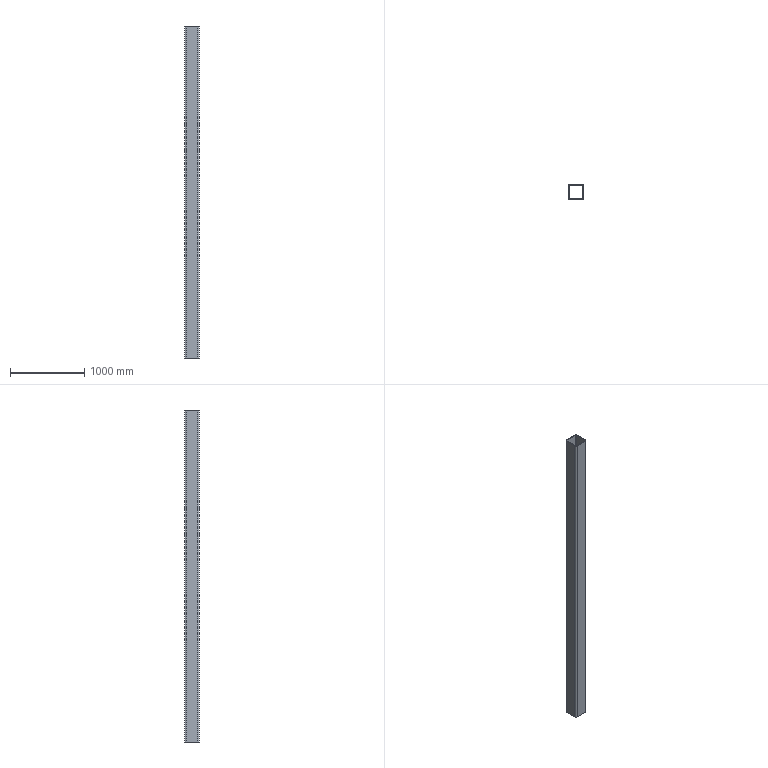Part | SolidWorks | features Extrusion 1 | 1 solid | 18 faces | box 200 x 200 x 4480 mm | volume 26540630 mm3 | plane 10 | cylinder 8 | commonest cylinder face diameters 24 x4 40 x4
STEP:
#1=CARTESIAN_POINT('',(-100.,-80.,4480.));
#2=VERTEX_POINT('',#1);
#3=CARTESIAN_POINT('',(-80.,-100.,4480.));
#4=VERTEX_POINT('',#3);
#5=CARTESIAN_POINT('',(-80.,-80.,4480.));
#6=DIRECTION('',(0.,0.,1.));
#7=DIRECTION('',(1.,0.,0.));
#8=AXIS2_PLACEMENT_3D('',#5,#6,#7);
#9=CIRCLE('',#8,20.);
#10=EDGE_CURVE('',#2,#4,#9,.T.);
#11=ORIENTED_EDGE('',*,*,#10,.T.);
#12=CARTESIAN_POINT('',(80.,-100.,4480.));
#13=VERTEX_POINT('',#12);
#14=CARTESIAN_POINT('',(-80.,-100.,4480.));
#15=DIRECTION('',(1.,0.,0.));
#16=VECTOR('',#15,1000.);
#17=LINE('',#14,#16);
#18=EDGE_CURVE('',#4,#13,#17,.T.);
#19=ORIENTED_EDGE('',*,*,#18,.T.);
#20=CARTESIAN_POINT('',(100.,-80.,4480.));
#21=VERTEX_POINT('',#20);
#22=CARTESIAN_POINT('',(80.,-80.,4480.));
#23=DIRECTION('',(0.,0.,1.));
#24=DIRECTION('',(1.,0.,0.));
#25=AXIS2_PLACEMENT_3D('',#22,#23,#24);
#26=CIRCLE('',#25,20.);
#27=EDGE_CURVE('',#13,#21,#26,.T.);
#28=ORIENTED_EDGE('',*,*,#27,.T.);
#29=CARTESIAN_POINT('',(100.,80.,4480.));
#30=VERTEX_POINT('',#29);
#31=CARTESIAN_POINT('',(100.,80.,4480.));
#32=DIRECTION('',(0.,1.,0.));
#33=VECTOR('',#32,1000.);
#34=LINE('',#31,#33);
#35=EDGE_CURVE('',#21,#30,#34,.T.);
#36=ORIENTED_EDGE('',*,*,#35,.T.);
#37=CARTESIAN_POINT('',(80.,100.,4480.));
#38=VERTEX_POINT('',#37);
#39=CARTESIAN_POINT('',(80.,80.,4480.));
#40=DIRECTION('',(0.,0.,1.));
#41=DIRECTION('',(-1.,0.,0.));
#42=AXIS2_PLACEMENT_3D('',#39,#40,#41);
#43=CIRCLE('',#42,20.);
#44=EDGE_CURVE('',#30,#38,#43,.T.);
#45=ORIENTED_EDGE('',*,*,#44,.T.);
#46=CARTESIAN_POINT('',(-80.,100.,4480.));
#47=VERTEX_POINT('',#46);
#48=CARTESIAN_POINT('',(-80.,100.,4480.));
#49=DIRECTION('',(-1.,0.,0.));
#50=VECTOR('',#49,1000.);
#51=LINE('',#48,#50);
#52=EDGE_CURVE('',#38,#47,#51,.T.);
#53=ORIENTED_EDGE('',*,*,#52,.T.);
#54=CARTESIAN_POINT('',(-100.,80.,4480.));
#55=VERTEX_POINT('',#54);
#56=CARTESIAN_POINT('',(-80.,80.,4480.));
#57=DIRECTION('',(0.,0.,1.));
#58=DIRECTION('',(1.,0.,0.));
#59=AXIS2_PLACEMENT_3D('',#56,#57,#58);
#60=CIRCLE('',#59,20.);
#61=EDGE_CURVE('',#47,#55,#60,.T.);
#62=ORIENTED_EDGE('',*,*,#61,.T.);
#63=CARTESIAN_POINT('',(-100.,80.,4480.));
#64=DIRECTION('',(0.,-1.,0.));
#65=VECTOR('',#64,1000.);
#66=LINE('',#63,#65);
#67=EDGE_CURVE('',#55,#2,#66,.T.);
#68=ORIENTED_EDGE('',*,*,#67,.T.);
#69=EDGE_LOOP('',(#11,#19,#28,#36,#45,#53,#62,#68));
#70=FACE_OUTER_BOUND('',#69,.T.);
#71=CARTESIAN_POINT('',(-92.,80.,4480.));
#72=VERTEX_POINT('',#71);
#73=CARTESIAN_POINT('',(-92.,-80.,4480.));
#74=VERTEX_POINT('',#73);
#75=CARTESIAN_POINT('',(-92.,80.,4480.));
#76=DIRECTION('',(0.,-1.,0.));
#77=VECTOR('',#76,1000.);
#78=LINE('',#75,#77);
#79=EDGE_CURVE('',#72,#74,#78,.T.);
#80=ORIENTED_EDGE('',*,*,#79,.F.);
#81=CARTESIAN_POINT('',(-80.,92.,4480.));
#82=VERTEX_POINT('',#81);
#83=CARTESIAN_POINT('',(-80.,80.,4480.));
#84=DIRECTION('',(0.,0.,1.));
#85=DIRECTION('',(1.,0.,0.));
#86=AXIS2_PLACEMENT_3D('',#83,#84,#85);
#87=CIRCLE('',#86,12.);
#88=EDGE_CURVE('',#82,#72,#87,.T.);
#89=ORIENTED_EDGE('',*,*,#88,.F.);
#90=CARTESIAN_POINT('',(80.,92.,4480.));
#91=VERTEX_POINT('',#90);
#92=CARTESIAN_POINT('',(-80.,92.,4480.));
#93=DIRECTION('',(-1.,0.,0.));
#94=VECTOR('',#93,1000.);
#95=LINE('',#92,#94);
#96=EDGE_CURVE('',#91,#82,#95,.T.);
#97=ORIENTED_EDGE('',*,*,#96,.F.);
#98=CARTESIAN_POINT('',(92.,80.,4480.));
#99=VERTEX_POINT('',#98);
#100=CARTESIAN_POINT('',(80.,80.,4480.));
#101=DIRECTION('',(0.,0.,1.));
#102=DIRECTION('',(-1.,0.,0.));
#103=AXIS2_PLACEMENT_3D('',#100,#101,#102);
#104=CIRCLE('',#103,12.);
#105=EDGE_CURVE('',#99,#91,#104,.T.);
#106=ORIENTED_EDGE('',*,*,#105,.F.);
#107=CARTESIAN_POINT('',(92.,-80.,4480.));
#108=VERTEX_POINT('',#107);
#109=CARTESIAN_POINT('',(92.,80.,4480.));
#110=DIRECTION('',(0.,1.,0.));
#111=VECTOR('',#110,1000.);
#112=LINE('',#109,#111);
#113=EDGE_CURVE('',#108,#99,#112,.T.);
#114=ORIENTED_EDGE('',*,*,#113,.F.);
#115=CARTESIAN_POINT('',(80.,-92.,4480.));
#116=VERTEX_POINT('',#115);
#117=CARTESIAN_POINT('',(80.,-80.,4480.));
#118=DIRECTION('',(0.,0.,1.));
#119=DIRECTION('',(1.,0.,0.));
#120=AXIS2_PLACEMENT_3D('',#117,#118,#119);
#121=CIRCLE('',#120,12.);
#122=EDGE_CURVE('',#116,#108,#121,.T.);
#123=ORIENTED_EDGE('',*,*,#122,.F.);
#124=CARTESIAN_POINT('',(-80.,-92.,4480.));
#125=VERTEX_POINT('',#124);
#126=CARTESIAN_POINT('',(-80.,-92.,4480.));
#127=DIRECTION('',(1.,0.,0.));
#128=VECTOR('',#127,1000.);
#129=LINE('',#126,#128);
#130=EDGE_CURVE('',#125,#116,#129,.T.);
#131=ORIENTED_EDGE('',*,*,#130,.F.);
#132=CARTESIAN_POINT('',(-80.,-80.,4480.));
#133=DIRECTION('',(0.,0.,1.));
#134=DIRECTION('',(1.,0.,0.));
#135=AXIS2_PLACEMENT_3D('',#132,#133,#134);
#136=CIRCLE('',#135,12.);
#137=EDGE_CURVE('',#74,#125,#136,.T.);
#138=ORIENTED_EDGE('',*,*,#137,.F.);
#139=EDGE_LOOP('',(#80,#89,#97,#106,#114,#123,#131,#138));
#140=FACE_BOUND('',#139,.T.);
#141=CARTESIAN_POINT('',(-80.,-80.,4480.));
#142=DIRECTION('',(0.,0.,1.));
#143=DIRECTION('',(1.,0.,0.));
#144=AXIS2_PLACEMENT_3D('',#141,#142,#143);
#145=PLANE('',#144);
#146=ADVANCED_FACE('',(#70,#140),#145,.T.);
#147=CARTESIAN_POINT('',(-100.,-80.,0.));
#148=VERTEX_POINT('',#147);
#149=CARTESIAN_POINT('',(-80.,-100.,0.));
#150=VERTEX_POINT('',#149);
#151=CARTESIAN_POINT('',(-80.,-80.,0.));
#152=DIRECTION('',(0.,0.,1.));
#153=DIRECTION('',(1.,0.,0.));
#154=AXIS2_PLACEMENT_3D('',#151,#152,#153);
#155=CIRCLE('',#154,20.);
#156=EDGE_CURVE('',#148,#150,#155,.T.);
#157=ORIENTED_EDGE('',*,*,#156,.F.);
#158=CARTESIAN_POINT('',(-100.,80.,0.));
#159=VERTEX_POINT('',#158);
#160=CARTESIAN_POINT('',(-100.,80.,0.));
#161=DIRECTION('',(0.,-1.,0.));
#162=VECTOR('',#161,1000.);
#163=LINE('',#160,#162);
#164=EDGE_CURVE('',#159,#148,#163,.T.);
#165=ORIENTED_EDGE('',*,*,#164,.F.);
#166=CARTESIAN_POINT('',(-80.,100.,0.));
#167=VERTEX_POINT('',#166);
#168=CARTESIAN_POINT('',(-80.,80.,0.));
#169=DIRECTION('',(0.,0.,1.));
#170=DIRECTION('',(1.,0.,0.));
#171=AXIS2_PLACEMENT_3D('',#168,#169,#170);
#172=CIRCLE('',#171,20.);
#173=EDGE_CURVE('',#167,#159,#172,.T.);
#174=ORIENTED_EDGE('',*,*,#173,.F.);
#175=CARTESIAN_POINT('',(80.,100.,0.));
#176=VERTEX_POINT('',#175);
#177=CARTESIAN_POINT('',(-80.,100.,0.));
#178=DIRECTION('',(-1.,0.,0.));
#179=VECTOR('',#178,1000.);
#180=LINE('',#177,#179);
#181=EDGE_CURVE('',#176,#167,#180,.T.);
#182=ORIENTED_EDGE('',*,*,#181,.F.);
#183=CARTESIAN_POINT('',(100.,80.,0.));
#184=VERTEX_POINT('',#183);
#185=CARTESIAN_POINT('',(80.,80.,0.));
#186=DIRECTION('',(0.,0.,1.));
#187=DIRECTION('',(-1.,0.,0.));
#188=AXIS2_PLACEMENT_3D('',#185,#186,#187);
#189=CIRCLE('',#188,20.);
#190=EDGE_CURVE('',#184,#176,#189,.T.);
#191=ORIENTED_EDGE('',*,*,#190,.F.);
#192=CARTESIAN_POINT('',(100.,-80.,0.));
#193=VERTEX_POINT('',#192);
#194=CARTESIAN_POINT('',(100.,80.,0.));
#195=DIRECTION('',(0.,1.,0.));
#196=VECTOR('',#195,1000.);
#197=LINE('',#194,#196);
#198=EDGE_CURVE('',#193,#184,#197,.T.);
#199=ORIENTED_EDGE('',*,*,#198,.F.);
#200=CARTESIAN_POINT('',(80.,-100.,0.));
#201=VERTEX_POINT('',#200);
#202=CARTESIAN_POINT('',(80.,-80.,0.));
#203=DIRECTION('',(0.,0.,1.));
#204=DIRECTION('',(1.,0.,0.));
#205=AXIS2_PLACEMENT_3D('',#202,#203,#204);
#206=CIRCLE('',#205,20.);
#207=EDGE_CURVE('',#201,#193,#206,.T.);
#208=ORIENTED_EDGE('',*,*,#207,.F.);
#209=CARTESIAN_POINT('',(-80.,-100.,0.));
#210=DIRECTION('',(1.,0.,0.));
#211=VECTOR('',#210,1000.);
#212=LINE('',#209,#211);
#213=EDGE_CURVE('',#150,#201,#212,.T.);
#214=ORIENTED_EDGE('',*,*,#213,.F.);
#215=EDGE_LOOP('',(#157,#165,#174,#182,#191,#199,#208,#214));
#216=FACE_OUTER_BOUND('',#215,.T.);
#217=CARTESIAN_POINT('',(-80.,92.,0.));
#218=VERTEX_POINT('',#217);
#219=CARTESIAN_POINT('',(-92.,80.,0.));
#220=VERTEX_POINT('',#219);
#221=CARTESIAN_POINT('',(-80.,80.,0.));
#222=DIRECTION('',(0.,0.,1.));
#223=DIRECTION('',(1.,0.,0.));
#224=AXIS2_PLACEMENT_3D('',#221,#222,#223);
#225=CIRCLE('',#224,12.);
#226=EDGE_CURVE('',#218,#220,#225,.T.);
#227=ORIENTED_EDGE('',*,*,#226,.T.);
#228=CARTESIAN_POINT('',(-92.,-80.,0.));
#229=VERTEX_POINT('',#228);
#230=CARTESIAN_POINT('',(-92.,80.,0.));
#231=DIRECTION('',(0.,-1.,0.));
#232=VECTOR('',#231,1000.);
#233=LINE('',#230,#232);
#234=EDGE_CURVE('',#220,#229,#233,.T.);
#235=ORIENTED_EDGE('',*,*,#234,.T.);
#236=CARTESIAN_POINT('',(-80.,-92.,0.));
#237=VERTEX_POINT('',#236);
#238=CARTESIAN_POINT('',(-80.,-80.,0.));
#239=DIRECTION('',(0.,0.,1.));
#240=DIRECTION('',(1.,0.,0.));
#241=AXIS2_PLACEMENT_3D('',#238,#239,#240);
#242=CIRCLE('',#241,12.);
#243=EDGE_CURVE('',#229,#237,#242,.T.);
#244=ORIENTED_EDGE('',*,*,#243,.T.);
#245=CARTESIAN_POINT('',(80.,-92.,0.));
#246=VERTEX_POINT('',#245);
#247=CARTESIAN_POINT('',(-80.,-92.,0.));
#248=DIRECTION('',(1.,0.,0.));
#249=VECTOR('',#248,1000.);
#250=LINE('',#247,#249);
#251=EDGE_CURVE('',#237,#246,#250,.T.);
#252=ORIENTED_EDGE('',*,*,#251,.T.);
#253=CARTESIAN_POINT('',(92.,-80.,0.));
#254=VERTEX_POINT('',#253);
#255=CARTESIAN_POINT('',(80.,-80.,0.));
#256=DIRECTION('',(0.,0.,1.));
#257=DIRECTION('',(1.,0.,0.));
#258=AXIS2_PLACEMENT_3D('',#255,#256,#257);
#259=CIRCLE('',#258,12.);
#260=EDGE_CURVE('',#246,#254,#259,.T.);
#261=ORIENTED_EDGE('',*,*,#260,.T.);
#262=CARTESIAN_POINT('',(92.,80.,0.));
#263=VERTEX_POINT('',#262);
#264=CARTESIAN_POINT('',(92.,80.,0.));
#265=DIRECTION('',(0.,1.,0.));
#266=VECTOR('',#265,1000.);
#267=LINE('',#264,#266);
#268=EDGE_CURVE('',#254,#263,#267,.T.);
#269=ORIENTED_EDGE('',*,*,#268,.T.);
#270=CARTESIAN_POINT('',(80.,92.,0.));
#271=VERTEX_POINT('',#270);
#272=CARTESIAN_POINT('',(80.,80.,0.));
#273=DIRECTION('',(0.,0.,1.));
#274=DIRECTION('',(-1.,0.,0.));
#275=AXIS2_PLACEMENT_3D('',#272,#273,#274);
#276=CIRCLE('',#275,12.);
#277=EDGE_CURVE('',#263,#271,#276,.T.);
#278=ORIENTED_EDGE('',*,*,#277,.T.);
#279=CARTESIAN_POINT('',(-80.,92.,0.));
#280=DIRECTION('',(-1.,0.,0.));
#281=VECTOR('',#280,1000.);
#282=LINE('',#279,#281);
#283=EDGE_CURVE('',#271,#218,#282,.T.);
#284=ORIENTED_EDGE('',*,*,#283,.T.);
#285=EDGE_LOOP('',(#227,#235,#244,#252,#261,#269,#278,#284));
#286=FACE_BOUND('',#285,.T.);
#287=CARTESIAN_POINT('',(-80.,-80.,0.));
#288=DIRECTION('',(0.,0.,1.));
#289=DIRECTION('',(1.,0.,0.));
#290=AXIS2_PLACEMENT_3D('',#287,#288,#289);
#291=PLANE('',#290);
#292=ADVANCED_FACE('',(#216,#286),#291,.F.);
#293=ORIENTED_EDGE('',*,*,#156,.T.);
#294=CARTESIAN_POINT('',(-80.,-100.,4480.));
#295=DIRECTION('',(0.,0.,-1.));
#296=VECTOR('',#295,1000.);
#297=LINE('',#294,#296);
#298=EDGE_CURVE('',#4,#150,#297,.T.);
#299=ORIENTED_EDGE('',*,*,#298,.F.);
#300=ORIENTED_EDGE('',*,*,#10,.F.);
#301=CARTESIAN_POINT('',(-100.,-80.,4480.));
#302=DIRECTION('',(0.,0.,-1.));
#303=VECTOR('',#302,1000.);
#304=LINE('',#301,#303);
#305=EDGE_CURVE('',#2,#148,#304,.T.);
#306=ORIENTED_EDGE('',*,*,#305,.T.);
#307=EDGE_LOOP('',(#293,#299,#300,#306));
#308=FACE_OUTER_BOUND('',#307,.T.);
#309=CARTESIAN_POINT('',(-80.,-80.,4480.));
#310=DIRECTION('',(0.,0.,-1.));
#311=DIRECTION('',(-1.,0.,0.));
#312=AXIS2_PLACEMENT_3D('',#309,#310,#311);
#313=CYLINDRICAL_SURFACE('',#312,20.);
#314=ADVANCED_FACE('',(#308),#313,.T.);
#315=ORIENTED_EDGE('',*,*,#213,.T.);
#316=CARTESIAN_POINT('',(80.,-100.,4480.));
#317=DIRECTION('',(0.,0.,-1.));
#318=VECTOR('',#317,1000.);
#319=LINE('',#316,#318);
#320=EDGE_CURVE('',#13,#201,#319,.T.);
#321=ORIENTED_EDGE('',*,*,#320,.F.);
#322=ORIENTED_EDGE('',*,*,#18,.F.);
#323=ORIENTED_EDGE('',*,*,#298,.T.);
#324=EDGE_LOOP('',(#315,#321,#322,#323));
#325=FACE_OUTER_BOUND('',#324,.T.);
#326=CARTESIAN_POINT('',(-80.,-100.,4480.));
#327=DIRECTION('',(0.,1.,0.));
#328=DIRECTION('',(0.,0.,1.));
#329=AXIS2_PLACEMENT_3D('',#326,#327,#328);
#330=PLANE('',#329);
#331=ADVANCED_FACE('',(#325),#330,.F.);
#332=ORIENTED_EDGE('',*,*,#207,.T.);
#333=CARTESIAN_POINT('',(100.,-80.,4480.));
#334=DIRECTION('',(0.,0.,-1.));
#335=VECTOR('',#334,1000.);
#336=LINE('',#333,#335);
#337=EDGE_CURVE('',#21,#193,#336,.T.);
#338=ORIENTED_EDGE('',*,*,#337,.F.);
#339=ORIENTED_EDGE('',*,*,#27,.F.);
#340=ORIENTED_EDGE('',*,*,#320,.T.);
#341=EDGE_LOOP('',(#332,#338,#339,#340));
#342=FACE_OUTER_BOUND('',#341,.T.);
#343=CARTESIAN_POINT('',(80.,-80.,4480.));
#344=DIRECTION('',(0.,0.,-1.));
#345=DIRECTION('',(-1.,0.,0.));
#346=AXIS2_PLACEMENT_3D('',#343,#344,#345);
#347=CYLINDRICAL_SURFACE('',#346,20.);
#348=ADVANCED_FACE('',(#342),#347,.T.);
#349=ORIENTED_EDGE('',*,*,#198,.T.);
#350=CARTESIAN_POINT('',(100.,80.,4480.));
#351=DIRECTION('',(0.,0.,-1.));
#352=VECTOR('',#351,1000.);
#353=LINE('',#350,#352);
#354=EDGE_CURVE('',#30,#184,#353,.T.);
#355=ORIENTED_EDGE('',*,*,#354,.F.);
#356=ORIENTED_EDGE('',*,*,#35,.F.);
#357=ORIENTED_EDGE('',*,*,#337,.T.);
#358=EDGE_LOOP('',(#349,#355,#356,#357));
#359=FACE_OUTER_BOUND('',#358,.T.);
#360=CARTESIAN_POINT('',(100.,80.,4480.));
#361=DIRECTION('',(-1.,0.,0.));
#362=DIRECTION('',(0.,-1.,0.));
#363=AXIS2_PLACEMENT_3D('',#360,#361,#362);
#364=PLANE('',#363);
#365=ADVANCED_FACE('',(#359),#364,.F.);
#366=ORIENTED_EDGE('',*,*,#190,.T.);
#367=CARTESIAN_POINT('',(80.,100.,4480.));
#368=DIRECTION('',(0.,0.,-1.));
#369=VECTOR('',#368,1000.);
#370=LINE('',#367,#369);
#371=EDGE_CURVE('',#38,#176,#370,.T.);
#372=ORIENTED_EDGE('',*,*,#371,.F.);
#373=ORIENTED_EDGE('',*,*,#44,.F.);
#374=ORIENTED_EDGE('',*,*,#354,.T.);
#375=EDGE_LOOP('',(#366,#372,#373,#374));
#376=FACE_OUTER_BOUND('',#375,.T.);
#377=CARTESIAN_POINT('',(80.,80.,4480.));
#378=DIRECTION('',(0.,0.,-1.));
#379=DIRECTION('',(-1.,0.,0.));
#380=AXIS2_PLACEMENT_3D('',#377,#378,#379);
#381=CYLINDRICAL_SURFACE('',#380,20.);
#382=ADVANCED_FACE('',(#376),#381,.T.);
#383=ORIENTED_EDGE('',*,*,#181,.T.);
#384=CARTESIAN_POINT('',(-80.,100.,4480.));
#385=DIRECTION('',(0.,0.,-1.));
#386=VECTOR('',#385,1000.);
#387=LINE('',#384,#386);
#388=EDGE_CURVE('',#47,#167,#387,.T.);
#389=ORIENTED_EDGE('',*,*,#388,.F.);
#390=ORIENTED_EDGE('',*,*,#52,.F.);
#391=ORIENTED_EDGE('',*,*,#371,.T.);
#392=EDGE_LOOP('',(#383,#389,#390,#391));
#393=FACE_OUTER_BOUND('',#392,.T.);
#394=CARTESIAN_POINT('',(-80.,100.,4480.));
#395=DIRECTION('',(0.,-1.,0.));
#396=DIRECTION('',(0.,0.,-1.));
#397=AXIS2_PLACEMENT_3D('',#394,#395,#396);
#398=PLANE('',#397);
#399=ADVANCED_FACE('',(#393),#398,.F.);
#400=ORIENTED_EDGE('',*,*,#173,.T.);
#401=CARTESIAN_POINT('',(-100.,80.,4480.));
#402=DIRECTION('',(0.,0.,-1.));
#403=VECTOR('',#402,1000.);
#404=LINE('',#401,#403);
#405=EDGE_CURVE('',#55,#159,#404,.T.);
#406=ORIENTED_EDGE('',*,*,#405,.F.);
#407=ORIENTED_EDGE('',*,*,#61,.F.);
#408=ORIENTED_EDGE('',*,*,#388,.T.);
#409=EDGE_LOOP('',(#400,#406,#407,#408));
#410=FACE_OUTER_BOUND('',#409,.T.);
#411=CARTESIAN_POINT('',(-80.,80.,4480.));
#412=DIRECTION('',(0.,0.,-1.));
#413=DIRECTION('',(-1.,0.,0.));
#414=AXIS2_PLACEMENT_3D('',#411,#412,#413);
#415=CYLINDRICAL_SURFACE('',#414,20.);
#416=ADVANCED_FACE('',(#410),#415,.T.);
#417=ORIENTED_EDGE('',*,*,#164,.T.);
#418=ORIENTED_EDGE('',*,*,#305,.F.);
#419=ORIENTED_EDGE('',*,*,#67,.F.);
#420=ORIENTED_EDGE('',*,*,#405,.T.);
#421=EDGE_LOOP('',(#417,#418,#419,#420));
#422=FACE_OUTER_BOUND('',#421,.T.);
#423=CARTESIAN_POINT('',(-100.,80.,4480.));
#424=DIRECTION('',(1.,0.,0.));
#425=DIRECTION('',(0.,1.,0.));
#426=AXIS2_PLACEMENT_3D('',#423,#424,#425);
#427=PLANE('',#426);
#428=ADVANCED_FACE('',(#422),#427,.F.);
#429=ORIENTED_EDGE('',*,*,#226,.F.);
#430=CARTESIAN_POINT('',(-80.,92.,4480.));
#431=DIRECTION('',(0.,0.,-1.));
#432=VECTOR('',#431,1000.);
#433=LINE('',#430,#432);
#434=EDGE_CURVE('',#82,#218,#433,.T.);
#435=ORIENTED_EDGE('',*,*,#434,.F.);
#436=ORIENTED_EDGE('',*,*,#88,.T.);
#437=CARTESIAN_POINT('',(-92.,80.,4480.));
#438=DIRECTION('',(0.,0.,-1.));
#439=VECTOR('',#438,1000.);
#440=LINE('',#437,#439);
#441=EDGE_CURVE('',#72,#220,#440,.T.);
#442=ORIENTED_EDGE('',*,*,#441,.T.);
#443=EDGE_LOOP('',(#429,#435,#436,#442));
#444=FACE_OUTER_BOUND('',#443,.T.);
#445=CARTESIAN_POINT('',(-80.,80.,4480.));
#446=DIRECTION('',(0.,0.,-1.));
#447=DIRECTION('',(-1.,0.,0.));
#448=AXIS2_PLACEMENT_3D('',#445,#446,#447);
#449=CYLINDRICAL_SURFACE('',#448,12.);
#450=ADVANCED_FACE('',(#444),#449,.F.);
#451=ORIENTED_EDGE('',*,*,#234,.F.);
#452=ORIENTED_EDGE('',*,*,#441,.F.);
#453=ORIENTED_EDGE('',*,*,#79,.T.);
#454=CARTESIAN_POINT('',(-92.,-80.,4480.));
#455=DIRECTION('',(0.,0.,-1.));
#456=VECTOR('',#455,1000.);
#457=LINE('',#454,#456);
#458=EDGE_CURVE('',#74,#229,#457,.T.);
#459=ORIENTED_EDGE('',*,*,#458,.T.);
#460=EDGE_LOOP('',(#451,#452,#453,#459));
#461=FACE_OUTER_BOUND('',#460,.T.);
#462=CARTESIAN_POINT('',(-92.,80.,4480.));
#463=DIRECTION('',(1.,0.,0.));
#464=DIRECTION('',(0.,0.,-1.));
#465=AXIS2_PLACEMENT_3D('',#462,#463,#464);
#466=PLANE('',#465);
#467=ADVANCED_FACE('',(#461),#466,.T.);
#468=ORIENTED_EDGE('',*,*,#243,.F.);
#469=ORIENTED_EDGE('',*,*,#458,.F.);
#470=ORIENTED_EDGE('',*,*,#137,.T.);
#471=CARTESIAN_POINT('',(-80.,-92.,4480.));
#472=DIRECTION('',(0.,0.,-1.));
#473=VECTOR('',#472,1000.);
#474=LINE('',#471,#473);
#475=EDGE_CURVE('',#125,#237,#474,.T.);
#476=ORIENTED_EDGE('',*,*,#475,.T.);
#477=EDGE_LOOP('',(#468,#469,#470,#476));
#478=FACE_OUTER_BOUND('',#477,.T.);
#479=CARTESIAN_POINT('',(-80.,-80.,4480.));
#480=DIRECTION('',(0.,0.,-1.));
#481=DIRECTION('',(-1.,0.,0.));
#482=AXIS2_PLACEMENT_3D('',#479,#480,#481);
#483=CYLINDRICAL_SURFACE('',#482,12.);
#484=ADVANCED_FACE('',(#478),#483,.F.);
#485=ORIENTED_EDGE('',*,*,#251,.F.);
#486=ORIENTED_EDGE('',*,*,#475,.F.);
#487=ORIENTED_EDGE('',*,*,#130,.T.);
#488=CARTESIAN_POINT('',(80.,-92.,4480.));
#489=DIRECTION('',(0.,0.,-1.));
#490=VECTOR('',#489,1000.);
#491=LINE('',#488,#490);
#492=EDGE_CURVE('',#116,#246,#491,.T.);
#493=ORIENTED_EDGE('',*,*,#492,.T.);
#494=EDGE_LOOP('',(#485,#486,#487,#493));
#495=FACE_OUTER_BOUND('',#494,.T.);
#496=CARTESIAN_POINT('',(-80.,-92.,4480.));
#497=DIRECTION('',(0.,1.,0.));
#498=DIRECTION('',(0.,0.,1.));
#499=AXIS2_PLACEMENT_3D('',#496,#497,#498);
#500=PLANE('',#499);
#501=ADVANCED_FACE('',(#495),#500,.T.);
#502=ORIENTED_EDGE('',*,*,#260,.F.);
#503=ORIENTED_EDGE('',*,*,#492,.F.);
#504=ORIENTED_EDGE('',*,*,#122,.T.);
#505=CARTESIAN_POINT('',(92.,-80.,4480.));
#506=DIRECTION('',(0.,0.,-1.));
#507=VECTOR('',#506,1000.);
#508=LINE('',#505,#507);
#509=EDGE_CURVE('',#108,#254,#508,.T.);
#510=ORIENTED_EDGE('',*,*,#509,.T.);
#511=EDGE_LOOP('',(#502,#503,#504,#510));
#512=FACE_OUTER_BOUND('',#511,.T.);
#513=CARTESIAN_POINT('',(80.,-80.,4480.));
#514=DIRECTION('',(0.,0.,-1.));
#515=DIRECTION('',(-1.,0.,0.));
#516=AXIS2_PLACEMENT_3D('',#513,#514,#515);
#517=CYLINDRICAL_SURFACE('',#516,12.);
#518=ADVANCED_FACE('',(#512),#517,.F.);
#519=ORIENTED_EDGE('',*,*,#268,.F.);
#520=ORIENTED_EDGE('',*,*,#509,.F.);
#521=ORIENTED_EDGE('',*,*,#113,.T.);
#522=CARTESIAN_POINT('',(92.,80.,4480.));
#523=DIRECTION('',(0.,0.,-1.));
#524=VECTOR('',#523,1000.);
#525=LINE('',#522,#524);
#526=EDGE_CURVE('',#99,#263,#525,.T.);
#527=ORIENTED_EDGE('',*,*,#526,.T.);
#528=EDGE_LOOP('',(#519,#520,#521,#527));
#529=FACE_OUTER_BOUND('',#528,.T.);
#530=CARTESIAN_POINT('',(92.,80.,4480.));
#531=DIRECTION('',(-1.,0.,0.));
#532=DIRECTION('',(0.,-1.,0.));
#533=AXIS2_PLACEMENT_3D('',#530,#531,#532);
#534=PLANE('',#533);
#535=ADVANCED_FACE('',(#529),#534,.T.);
#536=ORIENTED_EDGE('',*,*,#277,.F.);
#537=ORIENTED_EDGE('',*,*,#526,.F.);
#538=ORIENTED_EDGE('',*,*,#105,.T.);
#539=CARTESIAN_POINT('',(80.,92.,4480.));
#540=DIRECTION('',(0.,0.,-1.));
#541=VECTOR('',#540,1000.);
#542=LINE('',#539,#541);
#543=EDGE_CURVE('',#91,#271,#542,.T.);
#544=ORIENTED_EDGE('',*,*,#543,.T.);
#545=EDGE_LOOP('',(#536,#537,#538,#544));
#546=FACE_OUTER_BOUND('',#545,.T.);
#547=CARTESIAN_POINT('',(80.,80.,4480.));
#548=DIRECTION('',(0.,0.,-1.));
#549=DIRECTION('',(-1.,0.,0.));
#550=AXIS2_PLACEMENT_3D('',#547,#548,#549);
#551=CYLINDRICAL_SURFACE('',#550,12.);
#552=ADVANCED_FACE('',(#546),#551,.F.);
#553=ORIENTED_EDGE('',*,*,#283,.F.);
#554=ORIENTED_EDGE('',*,*,#543,.F.);
#555=ORIENTED_EDGE('',*,*,#96,.T.);
#556=ORIENTED_EDGE('',*,*,#434,.T.);
#557=EDGE_LOOP('',(#553,#554,#555,#556));
#558=FACE_OUTER_BOUND('',#557,.T.);
#559=CARTESIAN_POINT('',(-80.,92.,4480.));
#560=DIRECTION('',(0.,-1.,0.));
#561=DIRECTION('',(0.,0.,-1.));
#562=AXIS2_PLACEMENT_3D('',#559,#560,#561);
#563=PLANE('',#562);
#564=ADVANCED_FACE('',(#558),#563,.T.);
#565=CLOSED_SHELL('',(#146,#292,#314,#331,#348,#365,#382,#399,#416,#428,#450,#467,#484,#501,#518,#535,#552,#564));
#566=MANIFOLD_SOLID_BREP('',#565);
#567=CARTESIAN_POINT('',(0.,0.,0.));
#568=DIRECTION('',(0.,0.,1.));
#569=DIRECTION('',(1.,0.,0.));
#570=AXIS2_PLACEMENT_3D('',#567,#568,#569);
#571=(LENGTH_UNIT()NAMED_UNIT(*)SI_UNIT(.MILLI.,.METRE.));
#572=UNCERTAINTY_MEASURE_WITH_UNIT(LENGTH_MEASURE(0.00001),#571,'','');
#573=(NAMED_UNIT(*)PLANE_ANGLE_UNIT()SI_UNIT($,.RADIAN.));
#574=(NAMED_UNIT(*)SI_UNIT($,.STERADIAN.)SOLID_ANGLE_UNIT());
#575=(GEOMETRIC_REPRESENTATION_CONTEXT(3)GLOBAL_UNCERTAINTY_ASSIGNED_CONTEXT((#572))GLOBAL_UNIT_ASSIGNED_CONTEXT((#571,#573,#574))REPRESENTATION_CONTEXT('',''));
#576=ADVANCED_BREP_SHAPE_REPRESENTATION('',(#566,#570),#575);